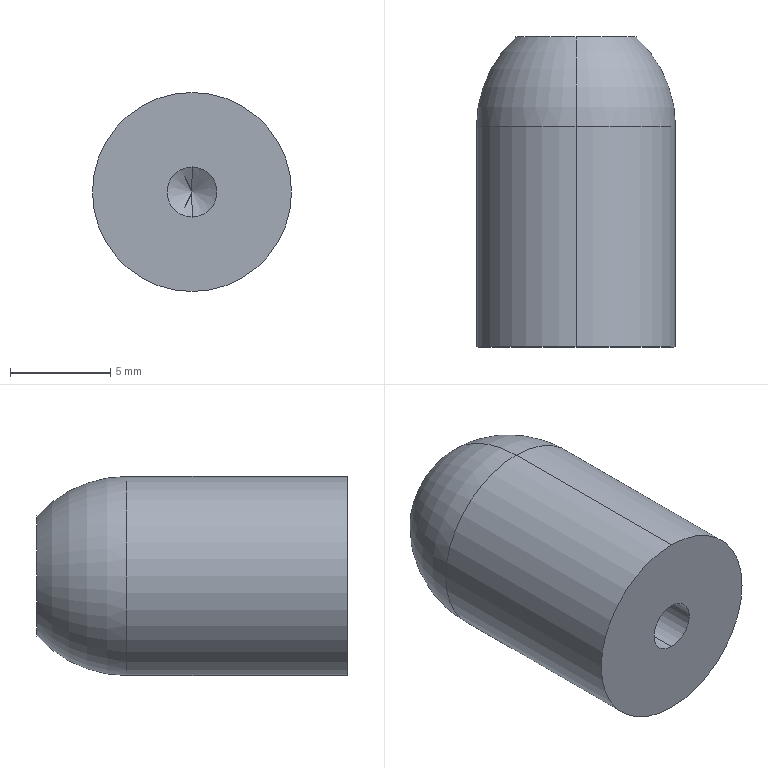Part | SolidWorks | features HoleWzd 1, Revolution 1 | 1 solid | 10 faces | box 9.95 x 15.5 x 9.95 mm | volume 1091 mm3 | cylinder 4 | cone 2 | plane 2 | torus 2 | commonest cylinder face diameters 2.5 x2 9.95 x2
STEP:
#1=CARTESIAN_POINT('',(0.,7.5,1.25));
#2=VERTEX_POINT('',#1);
#3=CARTESIAN_POINT('',(0.,7.5,-1.25));
#4=VERTEX_POINT('',#3);
#5=CARTESIAN_POINT('',(0.,7.5,0.));
#6=DIRECTION('',(0.,-1.,0.));
#7=DIRECTION('',(0.,0.,-1.));
#8=AXIS2_PLACEMENT_3D('',#5,#6,#7);
#9=CIRCLE('',#8,1.25);
#10=EDGE_CURVE('',#2,#4,#9,.T.);
#11=ORIENTED_EDGE('',*,*,#10,.F.);
#12=CARTESIAN_POINT('',(0.,0.,1.25));
#13=VERTEX_POINT('',#12);
#14=CARTESIAN_POINT('',(0.,0.,1.25));
#15=DIRECTION('',(0.,-1.,0.));
#16=VECTOR('',#15,1000.);
#17=LINE('',#14,#16);
#18=EDGE_CURVE('',#2,#13,#17,.T.);
#19=ORIENTED_EDGE('',*,*,#18,.T.);
#20=CARTESIAN_POINT('',(0.,0.,-1.25));
#21=VERTEX_POINT('',#20);
#22=CARTESIAN_POINT('',(0.,0.,0.));
#23=DIRECTION('',(0.,-1.,0.));
#24=DIRECTION('',(0.,0.,-1.));
#25=AXIS2_PLACEMENT_3D('',#22,#23,#24);
#26=CIRCLE('',#25,1.25);
#27=EDGE_CURVE('',#13,#21,#26,.T.);
#28=ORIENTED_EDGE('',*,*,#27,.T.);
#29=CARTESIAN_POINT('',(0.,0.,-1.25));
#30=DIRECTION('',(0.,-1.,0.));
#31=VECTOR('',#30,1000.);
#32=LINE('',#29,#31);
#33=EDGE_CURVE('',#4,#21,#32,.T.);
#34=ORIENTED_EDGE('',*,*,#33,.F.);
#35=EDGE_LOOP('',(#11,#19,#28,#34));
#36=FACE_OUTER_BOUND('',#35,.T.);
#37=CARTESIAN_POINT('',(0.,0.,0.));
#38=DIRECTION('',(0.,-1.,0.));
#39=DIRECTION('',(0.,0.,-1.));
#40=AXIS2_PLACEMENT_3D('',#37,#38,#39);
#41=CYLINDRICAL_SURFACE('',#40,1.25);
#42=ADVANCED_FACE('',(#36),#41,.F.);
#43=CARTESIAN_POINT('',(0.,8.251,0.));
#44=VERTEX_POINT('',#43);
#45=CARTESIAN_POINT('',(0.,7.5,-1.25));
#46=DIRECTION('',(0.,-0.515,-0.8572));
#47=VECTOR('',#46,1000.);
#48=LINE('',#45,#47);
#49=EDGE_CURVE('',#44,#4,#48,.T.);
#50=ORIENTED_EDGE('',*,*,#49,.F.);
#51=CARTESIAN_POINT('',(0.,7.5,1.25));
#52=DIRECTION('',(0.,-0.515,0.8572));
#53=VECTOR('',#52,1000.);
#54=LINE('',#51,#53);
#55=EDGE_CURVE('',#44,#2,#54,.T.);
#56=ORIENTED_EDGE('',*,*,#55,.T.);
#57=ORIENTED_EDGE('',*,*,#10,.T.);
#58=EDGE_LOOP('',(#50,#56,#57));
#59=FACE_OUTER_BOUND('',#58,.T.);
#60=CARTESIAN_POINT('',(0.,7.5,0.));
#61=DIRECTION('',(0.,-1.,0.));
#62=DIRECTION('',(0.,0.,-1.));
#63=AXIS2_PLACEMENT_3D('',#60,#61,#62);
#64=CONICAL_SURFACE('',#63,1.25,1.03);
#65=ADVANCED_FACE('',(#59),#64,.F.);
#66=CARTESIAN_POINT('',(0.,15.5,-3.));
#67=VERTEX_POINT('',#66);
#68=CARTESIAN_POINT('',(0.,15.5,3.));
#69=VERTEX_POINT('',#68);
#70=CARTESIAN_POINT('',(0.,15.5,0.));
#71=DIRECTION('',(0.,-1.,0.));
#72=DIRECTION('',(0.,0.,-1.));
#73=AXIS2_PLACEMENT_3D('',#70,#71,#72);
#74=CIRCLE('',#73,3.);
#75=EDGE_CURVE('',#67,#69,#74,.T.);
#76=ORIENTED_EDGE('',*,*,#75,.T.);
#77=CARTESIAN_POINT('',(0.,11.,4.975));
#78=VERTEX_POINT('',#77);
#79=CARTESIAN_POINT('',(0.,11.,-1.139));
#80=DIRECTION('',(1.,0.,0.));
#81=DIRECTION('',(0.,0.,-1.));
#82=AXIS2_PLACEMENT_3D('',#79,#80,#81);
#83=CIRCLE('',#82,6.114);
#84=EDGE_CURVE('',#69,#78,#83,.T.);
#85=ORIENTED_EDGE('',*,*,#84,.T.);
#86=CARTESIAN_POINT('',(0.,11.,-4.975));
#87=VERTEX_POINT('',#86);
#88=CARTESIAN_POINT('',(0.,11.,0.));
#89=DIRECTION('',(0.,-1.,0.));
#90=DIRECTION('',(0.,0.,-1.));
#91=AXIS2_PLACEMENT_3D('',#88,#89,#90);
#92=CIRCLE('',#91,4.975);
#93=EDGE_CURVE('',#87,#78,#92,.T.);
#94=ORIENTED_EDGE('',*,*,#93,.F.);
#95=CARTESIAN_POINT('',(0.,11.,1.139));
#96=DIRECTION('',(-1.,0.,0.));
#97=DIRECTION('',(0.,0.,1.));
#98=AXIS2_PLACEMENT_3D('',#95,#96,#97);
#99=CIRCLE('',#98,6.114);
#100=EDGE_CURVE('',#67,#87,#99,.T.);
#101=ORIENTED_EDGE('',*,*,#100,.F.);
#102=EDGE_LOOP('',(#76,#85,#94,#101));
#103=FACE_OUTER_BOUND('',#102,.T.);
#104=CARTESIAN_POINT('',(0.,11.,0.));
#105=DIRECTION('',(0.,-1.,0.));
#106=DIRECTION('',(0.,0.,-1.));
#107=AXIS2_PLACEMENT_3D('',#104,#105,#106);
#108=TOROIDAL_SURFACE('',#107,-1.139,6.114);
#109=ADVANCED_FACE('',(#103),#108,.T.);
#110=ORIENTED_EDGE('',*,*,#93,.T.);
#111=CARTESIAN_POINT('',(0.,0.,4.975));
#112=VERTEX_POINT('',#111);
#113=CARTESIAN_POINT('',(0.,0.,4.975));
#114=DIRECTION('',(0.,-1.,0.));
#115=VECTOR('',#114,1000.);
#116=LINE('',#113,#115);
#117=EDGE_CURVE('',#78,#112,#116,.T.);
#118=ORIENTED_EDGE('',*,*,#117,.T.);
#119=CARTESIAN_POINT('',(0.,0.,-4.975));
#120=VERTEX_POINT('',#119);
#121=CARTESIAN_POINT('',(0.,0.,0.));
#122=DIRECTION('',(0.,-1.,0.));
#123=DIRECTION('',(0.,0.,-1.));
#124=AXIS2_PLACEMENT_3D('',#121,#122,#123);
#125=CIRCLE('',#124,4.975);
#126=EDGE_CURVE('',#120,#112,#125,.T.);
#127=ORIENTED_EDGE('',*,*,#126,.F.);
#128=CARTESIAN_POINT('',(0.,0.,-4.975));
#129=DIRECTION('',(0.,-1.,0.));
#130=VECTOR('',#129,1000.);
#131=LINE('',#128,#130);
#132=EDGE_CURVE('',#87,#120,#131,.T.);
#133=ORIENTED_EDGE('',*,*,#132,.F.);
#134=EDGE_LOOP('',(#110,#118,#127,#133));
#135=FACE_OUTER_BOUND('',#134,.T.);
#136=CARTESIAN_POINT('',(0.,0.,0.));
#137=DIRECTION('',(0.,-1.,0.));
#138=DIRECTION('',(0.,0.,-1.));
#139=AXIS2_PLACEMENT_3D('',#136,#137,#138);
#140=CYLINDRICAL_SURFACE('',#139,4.975);
#141=ADVANCED_FACE('',(#135),#140,.T.);
#142=CARTESIAN_POINT('',(0.,0.,0.));
#143=DIRECTION('',(0.,-1.,0.));
#144=DIRECTION('',(0.,0.,-1.));
#145=AXIS2_PLACEMENT_3D('',#142,#143,#144);
#146=CIRCLE('',#145,1.25);
#147=EDGE_CURVE('',#21,#13,#146,.T.);
#148=ORIENTED_EDGE('',*,*,#147,.F.);
#149=ORIENTED_EDGE('',*,*,#27,.F.);
#150=EDGE_LOOP('',(#148,#149));
#151=FACE_BOUND('',#150,.T.);
#152=ORIENTED_EDGE('',*,*,#126,.T.);
#153=CARTESIAN_POINT('',(0.,0.,0.));
#154=DIRECTION('',(0.,-1.,0.));
#155=DIRECTION('',(0.,0.,-1.));
#156=AXIS2_PLACEMENT_3D('',#153,#154,#155);
#157=CIRCLE('',#156,4.975);
#158=EDGE_CURVE('',#112,#120,#157,.T.);
#159=ORIENTED_EDGE('',*,*,#158,.T.);
#160=EDGE_LOOP('',(#152,#159));
#161=FACE_OUTER_BOUND('',#160,.T.);
#162=CARTESIAN_POINT('',(0.,0.,0.));
#163=DIRECTION('',(0.,1.,0.));
#164=DIRECTION('',(0.,0.,1.));
#165=AXIS2_PLACEMENT_3D('',#162,#163,#164);
#166=PLANE('',#165);
#167=ADVANCED_FACE('',(#151,#161),#166,.F.);
#168=ORIENTED_EDGE('',*,*,#117,.F.);
#169=CARTESIAN_POINT('',(0.,11.,0.));
#170=DIRECTION('',(0.,-1.,0.));
#171=DIRECTION('',(0.,0.,-1.));
#172=AXIS2_PLACEMENT_3D('',#169,#170,#171);
#173=CIRCLE('',#172,4.975);
#174=EDGE_CURVE('',#78,#87,#173,.T.);
#175=ORIENTED_EDGE('',*,*,#174,.T.);
#176=ORIENTED_EDGE('',*,*,#132,.T.);
#177=ORIENTED_EDGE('',*,*,#158,.F.);
#178=EDGE_LOOP('',(#168,#175,#176,#177));
#179=FACE_OUTER_BOUND('',#178,.T.);
#180=CARTESIAN_POINT('',(0.,0.,0.));
#181=DIRECTION('',(0.,-1.,0.));
#182=DIRECTION('',(0.,0.,-1.));
#183=AXIS2_PLACEMENT_3D('',#180,#181,#182);
#184=CYLINDRICAL_SURFACE('',#183,4.975);
#185=ADVANCED_FACE('',(#179),#184,.T.);
#186=ORIENTED_EDGE('',*,*,#84,.F.);
#187=CARTESIAN_POINT('',(0.,15.5,0.));
#188=DIRECTION('',(0.,-1.,0.));
#189=DIRECTION('',(0.,0.,-1.));
#190=AXIS2_PLACEMENT_3D('',#187,#188,#189);
#191=CIRCLE('',#190,3.);
#192=EDGE_CURVE('',#69,#67,#191,.T.);
#193=ORIENTED_EDGE('',*,*,#192,.T.);
#194=ORIENTED_EDGE('',*,*,#100,.T.);
#195=ORIENTED_EDGE('',*,*,#174,.F.);
#196=EDGE_LOOP('',(#186,#193,#194,#195));
#197=FACE_OUTER_BOUND('',#196,.T.);
#198=CARTESIAN_POINT('',(0.,11.,0.));
#199=DIRECTION('',(0.,-1.,0.));
#200=DIRECTION('',(0.,0.,-1.));
#201=AXIS2_PLACEMENT_3D('',#198,#199,#200);
#202=TOROIDAL_SURFACE('',#201,-1.139,6.114);
#203=ADVANCED_FACE('',(#197),#202,.T.);
#204=ORIENTED_EDGE('',*,*,#75,.F.);
#205=ORIENTED_EDGE('',*,*,#192,.F.);
#206=EDGE_LOOP('',(#204,#205));
#207=FACE_OUTER_BOUND('',#206,.T.);
#208=CARTESIAN_POINT('',(-3.,15.5,0.));
#209=DIRECTION('',(0.,-1.,0.));
#210=DIRECTION('',(0.,0.,-1.));
#211=AXIS2_PLACEMENT_3D('',#208,#209,#210);
#212=PLANE('',#211);
#213=ADVANCED_FACE('',(#207),#212,.F.);
#214=ORIENTED_EDGE('',*,*,#55,.F.);
#215=ORIENTED_EDGE('',*,*,#49,.T.);
#216=CARTESIAN_POINT('',(0.,7.5,0.));
#217=DIRECTION('',(0.,-1.,0.));
#218=DIRECTION('',(0.,0.,-1.));
#219=AXIS2_PLACEMENT_3D('',#216,#217,#218);
#220=CIRCLE('',#219,1.25);
#221=EDGE_CURVE('',#4,#2,#220,.T.);
#222=ORIENTED_EDGE('',*,*,#221,.T.);
#223=EDGE_LOOP('',(#214,#215,#222));
#224=FACE_OUTER_BOUND('',#223,.T.);
#225=CARTESIAN_POINT('',(0.,7.5,0.));
#226=DIRECTION('',(0.,-1.,0.));
#227=DIRECTION('',(0.,0.,-1.));
#228=AXIS2_PLACEMENT_3D('',#225,#226,#227);
#229=CONICAL_SURFACE('',#228,1.25,1.03);
#230=ADVANCED_FACE('',(#224),#229,.F.);
#231=ORIENTED_EDGE('',*,*,#18,.F.);
#232=ORIENTED_EDGE('',*,*,#221,.F.);
#233=ORIENTED_EDGE('',*,*,#33,.T.);
#234=ORIENTED_EDGE('',*,*,#147,.T.);
#235=EDGE_LOOP('',(#231,#232,#233,#234));
#236=FACE_OUTER_BOUND('',#235,.T.);
#237=CARTESIAN_POINT('',(0.,0.,0.));
#238=DIRECTION('',(0.,-1.,0.));
#239=DIRECTION('',(0.,0.,-1.));
#240=AXIS2_PLACEMENT_3D('',#237,#238,#239);
#241=CYLINDRICAL_SURFACE('',#240,1.25);
#242=ADVANCED_FACE('',(#236),#241,.F.);
#243=CLOSED_SHELL('',(#42,#65,#109,#141,#167,#185,#203,#213,#230,#242));
#244=MANIFOLD_SOLID_BREP('',#243);
#245=CARTESIAN_POINT('',(0.,0.,0.));
#246=DIRECTION('',(0.,0.,1.));
#247=DIRECTION('',(1.,0.,0.));
#248=AXIS2_PLACEMENT_3D('',#245,#246,#247);
#249=(LENGTH_UNIT()NAMED_UNIT(*)SI_UNIT(.MILLI.,.METRE.));
#250=UNCERTAINTY_MEASURE_WITH_UNIT(LENGTH_MEASURE(0.00001),#249,'','');
#251=(NAMED_UNIT(*)PLANE_ANGLE_UNIT()SI_UNIT($,.RADIAN.));
#252=(NAMED_UNIT(*)SI_UNIT($,.STERADIAN.)SOLID_ANGLE_UNIT());
#253=(GEOMETRIC_REPRESENTATION_CONTEXT(3)GLOBAL_UNCERTAINTY_ASSIGNED_CONTEXT((#250))GLOBAL_UNIT_ASSIGNED_CONTEXT((#249,#251,#252))REPRESENTATION_CONTEXT('',''));
#254=ADVANCED_BREP_SHAPE_REPRESENTATION('',(#244,#248),#253);